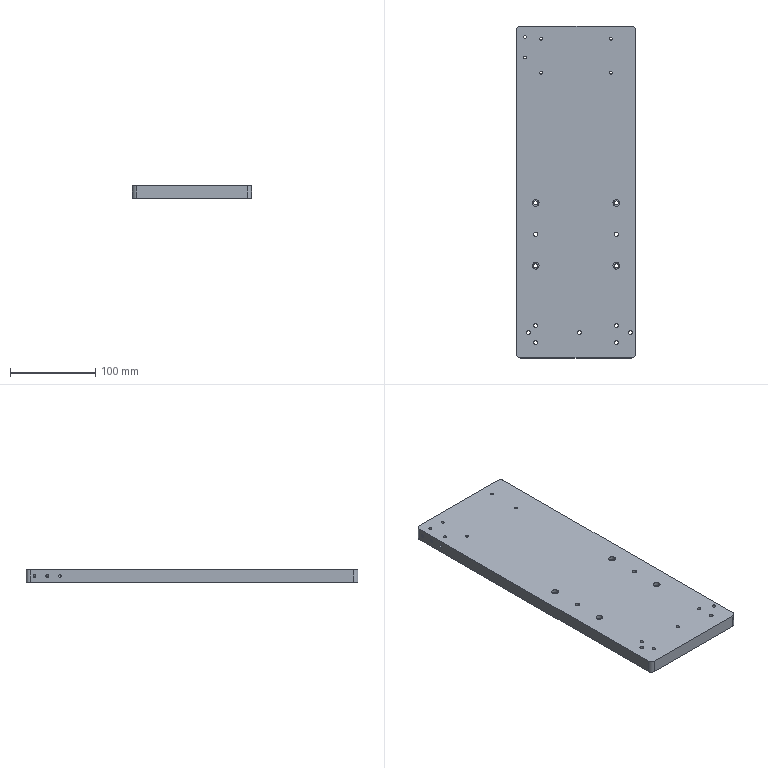Part | SolidWorks | features HoleWzd 7, Extrusion 1, Fillet 1, ICE 1 | 1 solid | 93 faces | box 140 x 390.5 x 15 mm | volume 813690 mm3 | cylinder 70 | plane 17 | cone 6 | commonest cylinder face diameters 4.5 x22 8 x22 3.3 x18 5 x4 10 x4